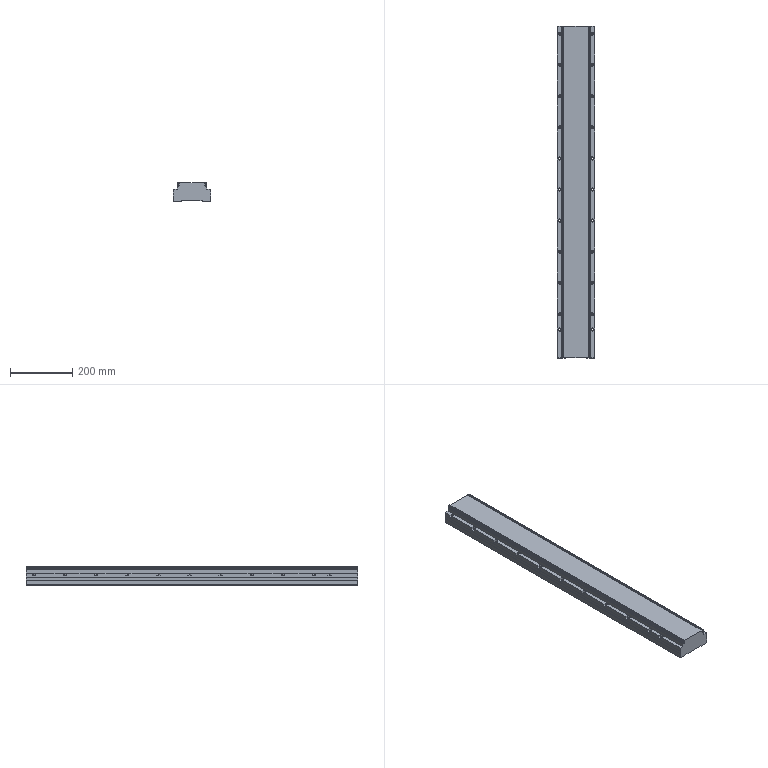Part | SolidWorks | features BaseBody 1 | 1 solid | 293 faces | box 120 x 1066 x 59 mm | volume 6777747 mm3 | plane 128 | cylinder 121 | cone 44 | commonest cylinder face diameters 6.8 x44 11 x33 1 x26 0.4 x6 6 x6 0.2 x2